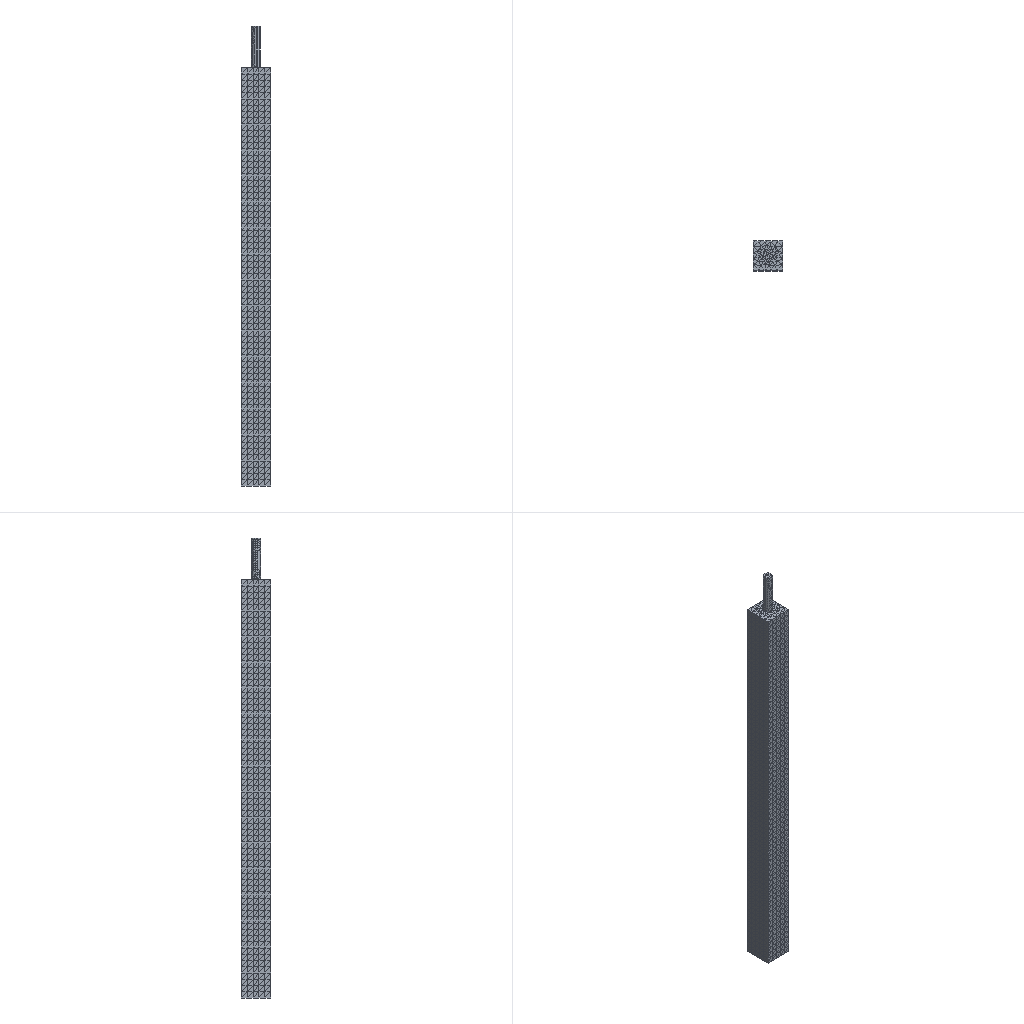Simulation study | abaqus
Set-up summary:
category,name,step,type,value,unit,region
solver,abaqus
solver,version,,,Abaqus/Standard 2020
units,not stated in the deck,,not stated
analysis,deck,,static,static
load_step,Step-1,Step-1,static
load_step,requested,,,1
mesh,nodes,,,61262
mesh,elements,,,37898
element_type,C3D10,,solid,37898
load,load commands in deck,,count,1
bc,support commands in deck,,count,3
material,MAO,,in results
material,SOIL,,in results
check,setup vs results,,match,"per instance, exact: element labels, types and connectivity; labels of the nodes the elements use; coordinates of those nodes at SINGLE_PRECISION in 2 of 2 instance(s)"
Abaqus input file, long lists of numbers shortened:
*Heading
** Job name: Job-1 Model name: Model-1
** Generated by: Abaqus/CAE 2020
*Preprint, echo=NO, model=NO, history=NO, contact=NO
**
** PARTS
**
*Part, name=merge-soil
*Node
      1,          35.,         -46.,         100.
      2,          35.,         -24.,         100.
** (26855 more lines like these left out)
*Element, type=C3D10
    1,  2126,  2127,  2128,  2129,  3879,  3878,  3877,  3881,  3880,  3882
    2,  2130,  2126,  2127,  2128,  3884,  3879,  3883,  3885,  3877,  3878
** (16981 more lines like these left out)
*Nset, nset=Set-3, generate
     1,  26857,      1
*Elset, elset=Set-3, generate
     1,  16983,      1
** Section: Section-1
*Solid Section, elset=Set-3, material=soil
,
*End Part
**
*Part, name=work
*Node
      1,   886.763,   1366.427,           5.
      2,   936.763,   1366.427,           5.
** (34403 more lines like these left out)
*Element, type=C3D10
   1, 3119, 3120, 3121, 3122, 5195, 5194, 5193, 5197, 5196, 5198
   2, 3119, 3123, 3122, 3124, 5200, 5199, 5197, 5202, 5201, 5203
** (20913 more lines like these left out)
*Nset, nset=Set-3, generate
     1,  34405,      1
*Elset, elset=Set-3, generate
     1,  20915,      1
** Section: Section-2
*Solid Section, elset=Set-3, material=mao
,
*End Part
**
**
** ASSEMBLY
**
*Assembly, name=Assembly
**
*Instance, name=work-1, part=work
35.,  -1412.428,  -786.763
35.,  -1412.428,  -786.763, 35., -1413.428,  -786.763, 90.
*End Instance
**
*Instance, name=merge-soil-1, part=merge-soil
*End Instance
**
*Node
      1,          35.,         -35.,        1100.
*Nset, nset=Set-2, instance=merge-soil-1
    83,    84,    88,    89,   502,   503,   504,   505,   654,   655,   656,   657,   658,   659,   660,   661
   662,   663,   664,   665,  1546,  1547,  1548,  1549,  1550,  1551,  1552,  1553,  1554,  1555,  1556,  1557
** (6 more lines like these left out)
*Elset, elset=Set-2, instance=merge-soil-1
  1882,  2006,  2241,  2283,  2537,  2730,  4460,  4577,  6483,  7418,  8813,  9370,  9471,  9565,  9616,  9617
  9697,  9761,  9767, 10562, 11885, 11908, 11946, 11967, 11992, 12003, 12027, 12034, 12049, 12050, 12051, 12060
** (2 more lines like these left out)
*Nset, nset=Set-3, instance=merge-soil-1
    81,    82,    83,    84,    87,    88,    89,    90,   436,   437,   438,   439,   440,   441,   442,   443
   444,   445,   446,   447,   448,   449,   450,   451,   452,   453,   454,   455,   456,   457,   458,   459
** (184 more lines like these left out)
*Elset, elset=Set-3, instance=merge-soil-1
   290,   925,  1974,  2078,  2117,  2238,  2250,  2263,  2268,  2270,  2281,  2285,  2295,  2317,  2323,  2383
  2384,  2411,  2412,  2435,  2461,  2474,  2499,  2509,  2519,  2531,  2540,  2581,  2625,  2649,  2672,  2675
** (82 more lines like these left out)
*Nset, nset=Set-4, instance=merge-soil-1
    81,    82,    83,    84,    87,    88,    89,    90,   432,   433,   434,   435,   436,   437,   438,   439
   440,   441,   442,   443,   444,   445,   446,   447,   448,   449,   450,   451,   452,   453,   454,   455
** (184 more lines like these left out)
*Elset, elset=Set-4, instance=merge-soil-1
   169,   253,   364,   438,   448,  1122,  1127,  1249,  1284,  1346,  1386,  1426,  1449,  1483,  1731,  1998
  2020,  2052,  2058,  2060,  2105,  2223,  2289,  2355,  2361,  2378,  2387,  2505,  2515,  2526,  2552,  2554
** (82 more lines like these left out)
*Nset, nset=Set-5
 1,
*Nset, nset=m_Set-1
 1,
*Elset, elset=_m_Surf-2_S3, internal, instance=work-1
    16,    31,    33,    36,    37,    43,    51,    77,   114,   122,   137,   184,   217,   220,   242,   263
   267,   273,   286,   287,   305,   326,   328,   333,   356,   375,   382,   386,   388,   397,   399,   411
** (253 more lines like these left out)
*Elset, elset=_m_Surf-2_S2, internal, instance=work-1
   874,  1188,  1271,  1350,  1376,  1553,  1578,  1580,  1596,  1628,  1629,  1635,  1714,  1795,  1800,  1887
  1899,  2095,  2106,  2137,  2278,  2593,  3147,  3220,  3276,  3295,  3324,  3365,  3377,  3390,  3409,  3421
** (51 more lines like these left out)
*Elset, elset=_m_Surf-2_S4, internal, instance=work-1
     3,    17,   488,   576,   677,   878,  1063,  1089,  1212,  1216,  1293,  1299,  1310,  1337,  1364,  1463
  1508,  1540,  1598,  1604,  1629,  1688,  1748,  1755,  1856,  1981,  2018,  2037,  2074,  2096,  2129,  2137
** (22 more lines like these left out)
*Elset, elset=_m_Surf-2_S1, internal, instance=work-1
    94,   427,   487,   557,   632,   677,   950,  1035,  1047,  1048,  1106,  1188,  1251,  1269,  1293,  1364
  1421,  1480,  1585,  1629,  1703,  1748,  1850,  1856,  2090,  2696,  2897,  2992,  3001,  3085,  3098,  3139
** (54 more lines like these left out)
*Surface, type=ELEMENT, name=m_Surf-2
_m_Surf-2_S3, S3
_m_Surf-2_S2, S2
_m_Surf-2_S4, S4
_m_Surf-2_S1, S1
*Elset, elset=_s_Surf-1_S3, internal, instance=work-1
  4332,  5944,  5949,  5980,  6411,  6437,  6447,  6458,  6462,  6464,  6465,  6476,  6477,  6483,  6490,  6492
  6494,  6655,  6656,  6657,  6658,  6661,  6665,  6673,  6674,  6675,  6690,  6697,  7362, 18644
*Elset, elset=_s_Surf-1_S4, internal, instance=work-1
 4674,
*Elset, elset=_s_Surf-1_S1, internal, instance=work-1
 7233,
*Surface, type=ELEMENT, name=s_Surf-1
_s_Surf-1_S3, S3
_s_Surf-1_S4, S4
_s_Surf-1_S1, S1
*Elset, elset=_s_Surf-2_S1, internal, instance=merge-soil-1
    28,   330,   441,   587,   845,   877,   927,  1310,  1456,  1700,  1933,  2121,  2309,  2665,  2705,  3036
  3114,  3117,  3154,  3236,  3261,  3328,  3369,  3713,  3827,  3840,  3947,  3988,  4070,  4085,  4579,  4789
** (3 more lines like these left out)
*Elset, elset=_s_Surf-2_S4, internal, instance=merge-soil-1
    68,   165,   190,   430,   564,   630,   632,   785,   927,   949,   997,  1008,  1192,  2121,  2123,  2753
  2836,  3006,  3061,  3128,  3141,  3149,  3232,  3240,  3307,  3327,  3328,  3330,  3404,  3522,  3565,  3791
** (6 more lines like these left out)
*Elset, elset=_s_Surf-2_S3, internal, instance=merge-soil-1
   885,  1457,  2003,  2038,  2059,  2123,  2130,  2133,  2164,  2172,  2195,  2197,  2220,  2340,  2347,  2403
  2517,  2522,  2528,  2532,  2533,  2541,  2555,  2558,  2572,  2632,  2644,  2653,  2665,  2688,  2698,  2702
** (68 more lines like these left out)
*Elset, elset=_s_Surf-2_S2, internal, instance=merge-soil-1
     5,   176,   318,   331,   332,   501,   730,   999,  1011,  2467,  2487,  2816,  3051,  3236,  3247,  3261
  3429,  3564,  3616,  3705,  3713,  3718,  3961,  4040,  4042,  4047,  4272,  4418,  4523,  4711,  4716,  4717
** (4 more lines like these left out)
*Surface, type=ELEMENT, name=s_Surf-2
_s_Surf-2_S1, S1
_s_Surf-2_S4, S4
_s_Surf-2_S2, S2
_s_Surf-2_S3, S3
** Constraint: Constraint-1
*Coupling, constraint name=Constraint-1, ref node=m_Set-1, surface=s_Surf-1
*Kinematic
*End Assembly
*Amplitude, name=Amp-1
             0.,              0.,              1.,              1.
**
** MATERIALS
**
*Material, name=mao
*Density
 7.8e-09,
*Elastic
210000., 0.3
*Plastic
300.,0.
*Material, name=soil
*Density
 2.7e-09,
*Elastic
24000., 0.23
*Mohr Coulomb
23., 0.1
*Mohr Coulomb Hardening
100.,0.
**
** INTERACTION PROPERTIES
**
*Surface Interaction, name=IntProp-1
1.,
*Friction, slip tolerance=0.005
 0.2,
*Surface Behavior, pressure-overclosure=HARD
**
** BOUNDARY CONDITIONS
**
** Name: BC-1 Type: 对称/反对称/完全固定
*Boundary
Set-2, ENCASTRE
** Name: BC-2 Type: 位移/转角
*Boundary
Set-3, 3, 3
** Name: BC-3 Type: 位移/转角
*Boundary
Set-4, 1, 1
**
** INTERACTIONS
**
** Interaction: Int-1
*Contact Pair, interaction=IntProp-1, type=SURFACE TO SURFACE
s_Surf-2, m_Surf-2
** ----------------------------------------------------------------
**
** STEP: Step-1
**
*Step, name=Step-1, nlgeom=YES, inc=1000
*Static, stabilize=0.0002, allsdtol=0.05, continue=NO
0.01, 1., 1e-05, 1.
**
** LOADS
**
** Name: Load-1   Type: Concentrated force
*Cload, amplitude=Amp-1
Set-5, 3, 100000.
**
** OUTPUT REQUESTS
**
*Restart, write, frequency=0
**
** FIELD OUTPUT: F-Output-1
**
*Output, field
*Node Output
CF, RF, RM, RT, TF, U, V
*Element Output, directions=YES
E, LE, MISES, MISESMAX, MISESONLY, PE, PEEQ, PEMAG, S, SF, SSAVG
*Contact Output
CDISP, CFORCE, CSTATUS, CSTRESS
**
** HISTORY OUTPUT: H-Output-1
**
*Output, history
*Node Output, nset=Set-5
U3, V3
*End Step
Results summary:
result,step,,partial,increments=33 time=0.8121/1.0
result,analysis,,,static
result,last_loadstep,,,1
result,primary field,,,U
result,reaction total,,FX,-32.32,model units
result,reaction total,,FY,-16.485,model units
result,reaction total,,FZ,-70138.919,model units